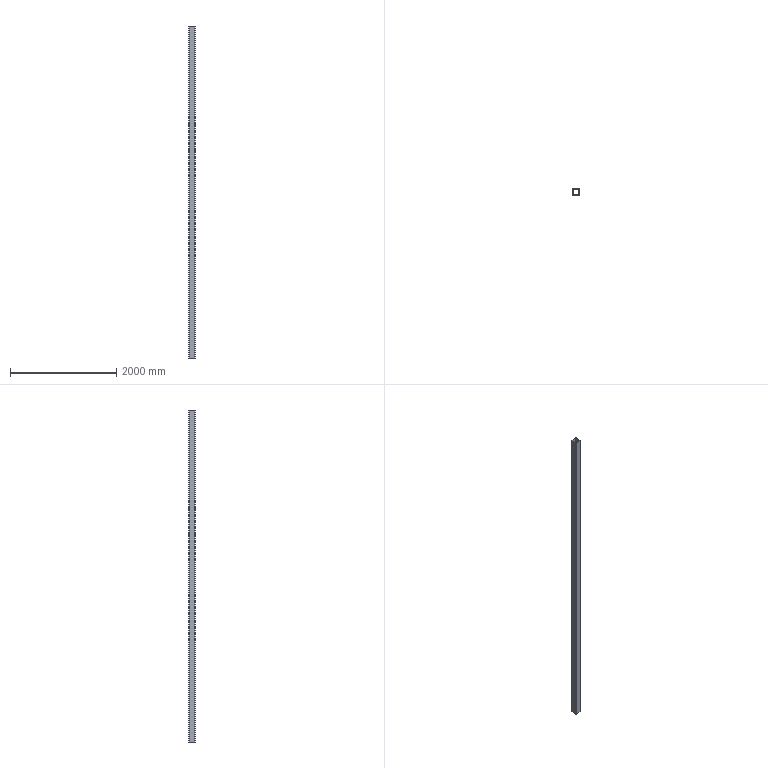Part | SolidWorks | features ICE 1, LibraryFeature 1 | 1 solid | 18 faces | box 120 x 120 x 6260 mm | volume 11360626 mm3 | plane 10 | cylinder 8 | commonest cylinder face diameters 8 x4 16 x4
STEP:
#1=CARTESIAN_POINT('',(52.,60.,-3130.));
#2=VERTEX_POINT('',#1);
#3=CARTESIAN_POINT('',(-52.,60.,-3130.));
#4=VERTEX_POINT('',#3);
#5=CARTESIAN_POINT('',(0.,60.,-3130.));
#6=DIRECTION('',(-1.,0.,0.));
#7=VECTOR('',#6,1000.);
#8=LINE('',#5,#7);
#9=EDGE_CURVE('',#2,#4,#8,.T.);
#10=ORIENTED_EDGE('',*,*,#9,.T.);
#11=CARTESIAN_POINT('',(-52.,60.,3130.));
#12=VERTEX_POINT('',#11);
#13=CARTESIAN_POINT('',(-52.,60.,3130.));
#14=DIRECTION('',(0.,0.,-1.));
#15=VECTOR('',#14,1000.);
#16=LINE('',#13,#15);
#17=EDGE_CURVE('',#12,#4,#16,.T.);
#18=ORIENTED_EDGE('',*,*,#17,.F.);
#19=CARTESIAN_POINT('',(52.,60.,3130.));
#20=VERTEX_POINT('',#19);
#21=CARTESIAN_POINT('',(0.,60.,3130.));
#22=DIRECTION('',(-1.,0.,0.));
#23=VECTOR('',#22,1000.);
#24=LINE('',#21,#23);
#25=EDGE_CURVE('',#20,#12,#24,.T.);
#26=ORIENTED_EDGE('',*,*,#25,.F.);
#27=CARTESIAN_POINT('',(52.,60.,3130.));
#28=DIRECTION('',(0.,0.,-1.));
#29=VECTOR('',#28,1000.);
#30=LINE('',#27,#29);
#31=EDGE_CURVE('',#20,#2,#30,.T.);
#32=ORIENTED_EDGE('',*,*,#31,.T.);
#33=EDGE_LOOP('',(#10,#18,#26,#32));
#34=FACE_OUTER_BOUND('',#33,.T.);
#35=CARTESIAN_POINT('',(0.,60.,3130.));
#36=DIRECTION('',(0.,-1.,0.));
#37=DIRECTION('',(0.,0.,-1.));
#38=AXIS2_PLACEMENT_3D('',#35,#36,#37);
#39=PLANE('',#38);
#40=ADVANCED_FACE('',(#34),#39,.F.);
#41=CARTESIAN_POINT('',(-60.,52.,-3130.));
#42=VERTEX_POINT('',#41);
#43=CARTESIAN_POINT('',(-52.,52.,-3130.));
#44=DIRECTION('',(0.,0.,1.));
#45=DIRECTION('',(1.,0.,0.));
#46=AXIS2_PLACEMENT_3D('',#43,#44,#45);
#47=CIRCLE('',#46,8.);
#48=EDGE_CURVE('',#4,#42,#47,.T.);
#49=ORIENTED_EDGE('',*,*,#48,.T.);
#50=CARTESIAN_POINT('',(-60.,52.,3130.));
#51=VERTEX_POINT('',#50);
#52=CARTESIAN_POINT('',(-60.,52.,3130.));
#53=DIRECTION('',(0.,0.,-1.));
#54=VECTOR('',#53,1000.);
#55=LINE('',#52,#54);
#56=EDGE_CURVE('',#51,#42,#55,.T.);
#57=ORIENTED_EDGE('',*,*,#56,.F.);
#58=CARTESIAN_POINT('',(-52.,52.,3130.));
#59=DIRECTION('',(0.,0.,1.));
#60=DIRECTION('',(1.,0.,0.));
#61=AXIS2_PLACEMENT_3D('',#58,#59,#60);
#62=CIRCLE('',#61,8.);
#63=EDGE_CURVE('',#12,#51,#62,.T.);
#64=ORIENTED_EDGE('',*,*,#63,.F.);
#65=ORIENTED_EDGE('',*,*,#17,.T.);
#66=EDGE_LOOP('',(#49,#57,#64,#65));
#67=FACE_OUTER_BOUND('',#66,.T.);
#68=CARTESIAN_POINT('',(-52.,52.,3130.));
#69=DIRECTION('',(0.,0.,-1.));
#70=DIRECTION('',(-1.,0.,0.));
#71=AXIS2_PLACEMENT_3D('',#68,#69,#70);
#72=CYLINDRICAL_SURFACE('',#71,8.);
#73=ADVANCED_FACE('',(#67),#72,.T.);
#74=CARTESIAN_POINT('',(-60.,-52.,-3130.));
#75=VERTEX_POINT('',#74);
#76=CARTESIAN_POINT('',(-60.,0.,-3130.));
#77=DIRECTION('',(0.,1.,0.));
#78=VECTOR('',#77,1000.);
#79=LINE('',#76,#78);
#80=EDGE_CURVE('',#75,#42,#79,.T.);
#81=ORIENTED_EDGE('',*,*,#80,.F.);
#82=CARTESIAN_POINT('',(-60.,-52.,3130.));
#83=VERTEX_POINT('',#82);
#84=CARTESIAN_POINT('',(-60.,-52.,3130.));
#85=DIRECTION('',(0.,0.,-1.));
#86=VECTOR('',#85,1000.);
#87=LINE('',#84,#86);
#88=EDGE_CURVE('',#83,#75,#87,.T.);
#89=ORIENTED_EDGE('',*,*,#88,.F.);
#90=CARTESIAN_POINT('',(-60.,0.,3130.));
#91=DIRECTION('',(0.,1.,0.));
#92=VECTOR('',#91,1000.);
#93=LINE('',#90,#92);
#94=EDGE_CURVE('',#83,#51,#93,.T.);
#95=ORIENTED_EDGE('',*,*,#94,.T.);
#96=ORIENTED_EDGE('',*,*,#56,.T.);
#97=EDGE_LOOP('',(#81,#89,#95,#96));
#98=FACE_OUTER_BOUND('',#97,.T.);
#99=CARTESIAN_POINT('',(-60.,0.,3130.));
#100=DIRECTION('',(-1.,0.,0.));
#101=DIRECTION('',(0.,0.,1.));
#102=AXIS2_PLACEMENT_3D('',#99,#100,#101);
#103=PLANE('',#102);
#104=ADVANCED_FACE('',(#98),#103,.T.);
#105=CARTESIAN_POINT('',(-52.,-60.,-3130.));
#106=VERTEX_POINT('',#105);
#107=CARTESIAN_POINT('',(-52.,-52.,-3130.));
#108=DIRECTION('',(0.,0.,1.));
#109=DIRECTION('',(1.,0.,0.));
#110=AXIS2_PLACEMENT_3D('',#107,#108,#109);
#111=CIRCLE('',#110,8.);
#112=EDGE_CURVE('',#75,#106,#111,.T.);
#113=ORIENTED_EDGE('',*,*,#112,.T.);
#114=CARTESIAN_POINT('',(-52.,-60.,3130.));
#115=VERTEX_POINT('',#114);
#116=CARTESIAN_POINT('',(-52.,-60.,3130.));
#117=DIRECTION('',(0.,0.,-1.));
#118=VECTOR('',#117,1000.);
#119=LINE('',#116,#118);
#120=EDGE_CURVE('',#115,#106,#119,.T.);
#121=ORIENTED_EDGE('',*,*,#120,.F.);
#122=CARTESIAN_POINT('',(-52.,-52.,3130.));
#123=DIRECTION('',(0.,0.,1.));
#124=DIRECTION('',(1.,0.,0.));
#125=AXIS2_PLACEMENT_3D('',#122,#123,#124);
#126=CIRCLE('',#125,8.);
#127=EDGE_CURVE('',#83,#115,#126,.T.);
#128=ORIENTED_EDGE('',*,*,#127,.F.);
#129=ORIENTED_EDGE('',*,*,#88,.T.);
#130=EDGE_LOOP('',(#113,#121,#128,#129));
#131=FACE_OUTER_BOUND('',#130,.T.);
#132=CARTESIAN_POINT('',(-52.,-52.,3130.));
#133=DIRECTION('',(0.,0.,-1.));
#134=DIRECTION('',(-1.,0.,0.));
#135=AXIS2_PLACEMENT_3D('',#132,#133,#134);
#136=CYLINDRICAL_SURFACE('',#135,8.);
#137=ADVANCED_FACE('',(#131),#136,.T.);
#138=CARTESIAN_POINT('',(52.,-60.,-3130.));
#139=VERTEX_POINT('',#138);
#140=CARTESIAN_POINT('',(0.,-60.,-3130.));
#141=DIRECTION('',(1.,0.,0.));
#142=VECTOR('',#141,1000.);
#143=LINE('',#140,#142);
#144=EDGE_CURVE('',#106,#139,#143,.T.);
#145=ORIENTED_EDGE('',*,*,#144,.T.);
#146=CARTESIAN_POINT('',(52.,-60.,3130.));
#147=VERTEX_POINT('',#146);
#148=CARTESIAN_POINT('',(52.,-60.,3130.));
#149=DIRECTION('',(0.,0.,-1.));
#150=VECTOR('',#149,1000.);
#151=LINE('',#148,#150);
#152=EDGE_CURVE('',#147,#139,#151,.T.);
#153=ORIENTED_EDGE('',*,*,#152,.F.);
#154=CARTESIAN_POINT('',(0.,-60.,3130.));
#155=DIRECTION('',(1.,0.,0.));
#156=VECTOR('',#155,1000.);
#157=LINE('',#154,#156);
#158=EDGE_CURVE('',#115,#147,#157,.T.);
#159=ORIENTED_EDGE('',*,*,#158,.F.);
#160=ORIENTED_EDGE('',*,*,#120,.T.);
#161=EDGE_LOOP('',(#145,#153,#159,#160));
#162=FACE_OUTER_BOUND('',#161,.T.);
#163=CARTESIAN_POINT('',(0.,-60.,3130.));
#164=DIRECTION('',(0.,1.,0.));
#165=DIRECTION('',(0.,0.,1.));
#166=AXIS2_PLACEMENT_3D('',#163,#164,#165);
#167=PLANE('',#166);
#168=ADVANCED_FACE('',(#162),#167,.F.);
#169=CARTESIAN_POINT('',(60.,-52.,-3130.));
#170=VERTEX_POINT('',#169);
#171=CARTESIAN_POINT('',(52.,-52.,-3130.));
#172=DIRECTION('',(0.,0.,1.));
#173=DIRECTION('',(1.,0.,0.));
#174=AXIS2_PLACEMENT_3D('',#171,#172,#173);
#175=CIRCLE('',#174,8.);
#176=EDGE_CURVE('',#139,#170,#175,.T.);
#177=ORIENTED_EDGE('',*,*,#176,.T.);
#178=CARTESIAN_POINT('',(60.,-52.,3130.));
#179=VERTEX_POINT('',#178);
#180=CARTESIAN_POINT('',(60.,-52.,3130.));
#181=DIRECTION('',(0.,0.,-1.));
#182=VECTOR('',#181,1000.);
#183=LINE('',#180,#182);
#184=EDGE_CURVE('',#179,#170,#183,.T.);
#185=ORIENTED_EDGE('',*,*,#184,.F.);
#186=CARTESIAN_POINT('',(52.,-52.,3130.));
#187=DIRECTION('',(0.,0.,1.));
#188=DIRECTION('',(1.,0.,0.));
#189=AXIS2_PLACEMENT_3D('',#186,#187,#188);
#190=CIRCLE('',#189,8.);
#191=EDGE_CURVE('',#147,#179,#190,.T.);
#192=ORIENTED_EDGE('',*,*,#191,.F.);
#193=ORIENTED_EDGE('',*,*,#152,.T.);
#194=EDGE_LOOP('',(#177,#185,#192,#193));
#195=FACE_OUTER_BOUND('',#194,.T.);
#196=CARTESIAN_POINT('',(52.,-52.,3130.));
#197=DIRECTION('',(0.,0.,-1.));
#198=DIRECTION('',(-1.,0.,0.));
#199=AXIS2_PLACEMENT_3D('',#196,#197,#198);
#200=CYLINDRICAL_SURFACE('',#199,8.);
#201=ADVANCED_FACE('',(#195),#200,.T.);
#202=CARTESIAN_POINT('',(60.,52.,-3130.));
#203=VERTEX_POINT('',#202);
#204=CARTESIAN_POINT('',(60.,0.,-3130.));
#205=DIRECTION('',(0.,-1.,0.));
#206=VECTOR('',#205,1000.);
#207=LINE('',#204,#206);
#208=EDGE_CURVE('',#203,#170,#207,.T.);
#209=ORIENTED_EDGE('',*,*,#208,.F.);
#210=CARTESIAN_POINT('',(60.,52.,3130.));
#211=VERTEX_POINT('',#210);
#212=CARTESIAN_POINT('',(60.,52.,3130.));
#213=DIRECTION('',(0.,0.,-1.));
#214=VECTOR('',#213,1000.);
#215=LINE('',#212,#214);
#216=EDGE_CURVE('',#211,#203,#215,.T.);
#217=ORIENTED_EDGE('',*,*,#216,.F.);
#218=CARTESIAN_POINT('',(60.,0.,3130.));
#219=DIRECTION('',(0.,-1.,0.));
#220=VECTOR('',#219,1000.);
#221=LINE('',#218,#220);
#222=EDGE_CURVE('',#211,#179,#221,.T.);
#223=ORIENTED_EDGE('',*,*,#222,.T.);
#224=ORIENTED_EDGE('',*,*,#184,.T.);
#225=EDGE_LOOP('',(#209,#217,#223,#224));
#226=FACE_OUTER_BOUND('',#225,.T.);
#227=CARTESIAN_POINT('',(60.,0.,3130.));
#228=DIRECTION('',(1.,0.,0.));
#229=DIRECTION('',(0.,0.,-1.));
#230=AXIS2_PLACEMENT_3D('',#227,#228,#229);
#231=PLANE('',#230);
#232=ADVANCED_FACE('',(#226),#231,.T.);
#233=CARTESIAN_POINT('',(-56.,-52.,-3130.));
#234=VERTEX_POINT('',#233);
#235=CARTESIAN_POINT('',(-52.,-56.,-3130.));
#236=VERTEX_POINT('',#235);
#237=CARTESIAN_POINT('',(-52.,-52.,-3130.));
#238=DIRECTION('',(0.,0.,1.));
#239=DIRECTION('',(1.,0.,0.));
#240=AXIS2_PLACEMENT_3D('',#237,#238,#239);
#241=CIRCLE('',#240,4.);
#242=EDGE_CURVE('',#234,#236,#241,.T.);
#243=ORIENTED_EDGE('',*,*,#242,.F.);
#244=CARTESIAN_POINT('',(-56.,-52.,3130.));
#245=VERTEX_POINT('',#244);
#246=CARTESIAN_POINT('',(-56.,-52.,3130.));
#247=DIRECTION('',(0.,0.,-1.));
#248=VECTOR('',#247,1000.);
#249=LINE('',#246,#248);
#250=EDGE_CURVE('',#245,#234,#249,.T.);
#251=ORIENTED_EDGE('',*,*,#250,.F.);
#252=CARTESIAN_POINT('',(-52.,-56.,3130.));
#253=VERTEX_POINT('',#252);
#254=CARTESIAN_POINT('',(-52.,-52.,3130.));
#255=DIRECTION('',(0.,0.,1.));
#256=DIRECTION('',(1.,0.,0.));
#257=AXIS2_PLACEMENT_3D('',#254,#255,#256);
#258=CIRCLE('',#257,4.);
#259=EDGE_CURVE('',#245,#253,#258,.T.);
#260=ORIENTED_EDGE('',*,*,#259,.T.);
#261=CARTESIAN_POINT('',(-52.,-56.,3130.));
#262=DIRECTION('',(0.,0.,-1.));
#263=VECTOR('',#262,1000.);
#264=LINE('',#261,#263);
#265=EDGE_CURVE('',#253,#236,#264,.T.);
#266=ORIENTED_EDGE('',*,*,#265,.T.);
#267=EDGE_LOOP('',(#243,#251,#260,#266));
#268=FACE_OUTER_BOUND('',#267,.T.);
#269=CARTESIAN_POINT('',(-52.,-52.,3130.));
#270=DIRECTION('',(0.,0.,-1.));
#271=DIRECTION('',(-1.,0.,0.));
#272=AXIS2_PLACEMENT_3D('',#269,#270,#271);
#273=CYLINDRICAL_SURFACE('',#272,4.);
#274=ADVANCED_FACE('',(#268),#273,.F.);
#275=CARTESIAN_POINT('',(-56.,52.,-3130.));
#276=VERTEX_POINT('',#275);
#277=CARTESIAN_POINT('',(-56.,0.,-3130.));
#278=DIRECTION('',(0.,1.,0.));
#279=VECTOR('',#278,1000.);
#280=LINE('',#277,#279);
#281=EDGE_CURVE('',#234,#276,#280,.T.);
#282=ORIENTED_EDGE('',*,*,#281,.T.);
#283=CARTESIAN_POINT('',(-56.,52.,3130.));
#284=VERTEX_POINT('',#283);
#285=CARTESIAN_POINT('',(-56.,52.,3130.));
#286=DIRECTION('',(0.,0.,-1.));
#287=VECTOR('',#286,1000.);
#288=LINE('',#285,#287);
#289=EDGE_CURVE('',#284,#276,#288,.T.);
#290=ORIENTED_EDGE('',*,*,#289,.F.);
#291=CARTESIAN_POINT('',(-56.,0.,3130.));
#292=DIRECTION('',(0.,1.,0.));
#293=VECTOR('',#292,1000.);
#294=LINE('',#291,#293);
#295=EDGE_CURVE('',#245,#284,#294,.T.);
#296=ORIENTED_EDGE('',*,*,#295,.F.);
#297=ORIENTED_EDGE('',*,*,#250,.T.);
#298=EDGE_LOOP('',(#282,#290,#296,#297));
#299=FACE_OUTER_BOUND('',#298,.T.);
#300=CARTESIAN_POINT('',(-56.,0.,3130.));
#301=DIRECTION('',(-1.,0.,0.));
#302=DIRECTION('',(0.,0.,1.));
#303=AXIS2_PLACEMENT_3D('',#300,#301,#302);
#304=PLANE('',#303);
#305=ADVANCED_FACE('',(#299),#304,.F.);
#306=CARTESIAN_POINT('',(-52.,56.,-3130.));
#307=VERTEX_POINT('',#306);
#308=CARTESIAN_POINT('',(-52.,52.,-3130.));
#309=DIRECTION('',(0.,0.,1.));
#310=DIRECTION('',(1.,0.,0.));
#311=AXIS2_PLACEMENT_3D('',#308,#309,#310);
#312=CIRCLE('',#311,4.);
#313=EDGE_CURVE('',#307,#276,#312,.T.);
#314=ORIENTED_EDGE('',*,*,#313,.F.);
#315=CARTESIAN_POINT('',(-52.,56.,3130.));
#316=VERTEX_POINT('',#315);
#317=CARTESIAN_POINT('',(-52.,56.,3130.));
#318=DIRECTION('',(0.,0.,-1.));
#319=VECTOR('',#318,1000.);
#320=LINE('',#317,#319);
#321=EDGE_CURVE('',#316,#307,#320,.T.);
#322=ORIENTED_EDGE('',*,*,#321,.F.);
#323=CARTESIAN_POINT('',(-52.,52.,3130.));
#324=DIRECTION('',(0.,0.,1.));
#325=DIRECTION('',(1.,0.,0.));
#326=AXIS2_PLACEMENT_3D('',#323,#324,#325);
#327=CIRCLE('',#326,4.);
#328=EDGE_CURVE('',#316,#284,#327,.T.);
#329=ORIENTED_EDGE('',*,*,#328,.T.);
#330=ORIENTED_EDGE('',*,*,#289,.T.);
#331=EDGE_LOOP('',(#314,#322,#329,#330));
#332=FACE_OUTER_BOUND('',#331,.T.);
#333=CARTESIAN_POINT('',(-52.,52.,3130.));
#334=DIRECTION('',(0.,0.,-1.));
#335=DIRECTION('',(-1.,0.,0.));
#336=AXIS2_PLACEMENT_3D('',#333,#334,#335);
#337=CYLINDRICAL_SURFACE('',#336,4.);
#338=ADVANCED_FACE('',(#332),#337,.F.);
#339=CARTESIAN_POINT('',(52.,56.,-3130.));
#340=VERTEX_POINT('',#339);
#341=CARTESIAN_POINT('',(0.,56.,-3130.));
#342=DIRECTION('',(-1.,0.,0.));
#343=VECTOR('',#342,1000.);
#344=LINE('',#341,#343);
#345=EDGE_CURVE('',#340,#307,#344,.T.);
#346=ORIENTED_EDGE('',*,*,#345,.F.);
#347=CARTESIAN_POINT('',(52.,56.,3130.));
#348=VERTEX_POINT('',#347);
#349=CARTESIAN_POINT('',(52.,56.,3130.));
#350=DIRECTION('',(0.,0.,-1.));
#351=VECTOR('',#350,1000.);
#352=LINE('',#349,#351);
#353=EDGE_CURVE('',#348,#340,#352,.T.);
#354=ORIENTED_EDGE('',*,*,#353,.F.);
#355=CARTESIAN_POINT('',(0.,56.,3130.));
#356=DIRECTION('',(-1.,0.,0.));
#357=VECTOR('',#356,1000.);
#358=LINE('',#355,#357);
#359=EDGE_CURVE('',#348,#316,#358,.T.);
#360=ORIENTED_EDGE('',*,*,#359,.T.);
#361=ORIENTED_EDGE('',*,*,#321,.T.);
#362=EDGE_LOOP('',(#346,#354,#360,#361));
#363=FACE_OUTER_BOUND('',#362,.T.);
#364=CARTESIAN_POINT('',(0.,56.,3130.));
#365=DIRECTION('',(0.,-1.,0.));
#366=DIRECTION('',(0.,0.,-1.));
#367=AXIS2_PLACEMENT_3D('',#364,#365,#366);
#368=PLANE('',#367);
#369=ADVANCED_FACE('',(#363),#368,.T.);
#370=CARTESIAN_POINT('',(56.,52.,-3130.));
#371=VERTEX_POINT('',#370);
#372=CARTESIAN_POINT('',(52.,52.,-3130.));
#373=DIRECTION('',(0.,0.,1.));
#374=DIRECTION('',(1.,0.,0.));
#375=AXIS2_PLACEMENT_3D('',#372,#373,#374);
#376=CIRCLE('',#375,4.);
#377=EDGE_CURVE('',#371,#340,#376,.T.);
#378=ORIENTED_EDGE('',*,*,#377,.F.);
#379=CARTESIAN_POINT('',(56.,52.,3130.));
#380=VERTEX_POINT('',#379);
#381=CARTESIAN_POINT('',(56.,52.,3130.));
#382=DIRECTION('',(0.,0.,-1.));
#383=VECTOR('',#382,1000.);
#384=LINE('',#381,#383);
#385=EDGE_CURVE('',#380,#371,#384,.T.);
#386=ORIENTED_EDGE('',*,*,#385,.F.);
#387=CARTESIAN_POINT('',(52.,52.,3130.));
#388=DIRECTION('',(0.,0.,1.));
#389=DIRECTION('',(1.,0.,0.));
#390=AXIS2_PLACEMENT_3D('',#387,#388,#389);
#391=CIRCLE('',#390,4.);
#392=EDGE_CURVE('',#380,#348,#391,.T.);
#393=ORIENTED_EDGE('',*,*,#392,.T.);
#394=ORIENTED_EDGE('',*,*,#353,.T.);
#395=EDGE_LOOP('',(#378,#386,#393,#394));
#396=FACE_OUTER_BOUND('',#395,.T.);
#397=CARTESIAN_POINT('',(52.,52.,3130.));
#398=DIRECTION('',(0.,0.,-1.));
#399=DIRECTION('',(-1.,0.,0.));
#400=AXIS2_PLACEMENT_3D('',#397,#398,#399);
#401=CYLINDRICAL_SURFACE('',#400,4.);
#402=ADVANCED_FACE('',(#396),#401,.F.);
#403=CARTESIAN_POINT('',(56.,-52.,-3130.));
#404=VERTEX_POINT('',#403);
#405=CARTESIAN_POINT('',(56.,0.,-3130.));
#406=DIRECTION('',(0.,-1.,0.));
#407=VECTOR('',#406,1000.);
#408=LINE('',#405,#407);
#409=EDGE_CURVE('',#371,#404,#408,.T.);
#410=ORIENTED_EDGE('',*,*,#409,.T.);
#411=CARTESIAN_POINT('',(56.,-52.,3130.));
#412=VERTEX_POINT('',#411);
#413=CARTESIAN_POINT('',(56.,-52.,3130.));
#414=DIRECTION('',(0.,0.,-1.));
#415=VECTOR('',#414,1000.);
#416=LINE('',#413,#415);
#417=EDGE_CURVE('',#412,#404,#416,.T.);
#418=ORIENTED_EDGE('',*,*,#417,.F.);
#419=CARTESIAN_POINT('',(56.,0.,3130.));
#420=DIRECTION('',(0.,-1.,0.));
#421=VECTOR('',#420,1000.);
#422=LINE('',#419,#421);
#423=EDGE_CURVE('',#380,#412,#422,.T.);
#424=ORIENTED_EDGE('',*,*,#423,.F.);
#425=ORIENTED_EDGE('',*,*,#385,.T.);
#426=EDGE_LOOP('',(#410,#418,#424,#425));
#427=FACE_OUTER_BOUND('',#426,.T.);
#428=CARTESIAN_POINT('',(56.,0.,3130.));
#429=DIRECTION('',(1.,0.,0.));
#430=DIRECTION('',(0.,0.,-1.));
#431=AXIS2_PLACEMENT_3D('',#428,#429,#430);
#432=PLANE('',#431);
#433=ADVANCED_FACE('',(#427),#432,.F.);
#434=CARTESIAN_POINT('',(52.,-56.,-3130.));
#435=VERTEX_POINT('',#434);
#436=CARTESIAN_POINT('',(52.,-52.,-3130.));
#437=DIRECTION('',(0.,0.,1.));
#438=DIRECTION('',(1.,0.,0.));
#439=AXIS2_PLACEMENT_3D('',#436,#437,#438);
#440=CIRCLE('',#439,4.);
#441=EDGE_CURVE('',#435,#404,#440,.T.);
#442=ORIENTED_EDGE('',*,*,#441,.F.);
#443=CARTESIAN_POINT('',(52.,-56.,3130.));
#444=VERTEX_POINT('',#443);
#445=CARTESIAN_POINT('',(52.,-56.,3130.));
#446=DIRECTION('',(0.,0.,-1.));
#447=VECTOR('',#446,1000.);
#448=LINE('',#445,#447);
#449=EDGE_CURVE('',#444,#435,#448,.T.);
#450=ORIENTED_EDGE('',*,*,#449,.F.);
#451=CARTESIAN_POINT('',(52.,-52.,3130.));
#452=DIRECTION('',(0.,0.,1.));
#453=DIRECTION('',(1.,0.,0.));
#454=AXIS2_PLACEMENT_3D('',#451,#452,#453);
#455=CIRCLE('',#454,4.);
#456=EDGE_CURVE('',#444,#412,#455,.T.);
#457=ORIENTED_EDGE('',*,*,#456,.T.);
#458=ORIENTED_EDGE('',*,*,#417,.T.);
#459=EDGE_LOOP('',(#442,#450,#457,#458));
#460=FACE_OUTER_BOUND('',#459,.T.);
#461=CARTESIAN_POINT('',(52.,-52.,3130.));
#462=DIRECTION('',(0.,0.,-1.));
#463=DIRECTION('',(-1.,0.,0.));
#464=AXIS2_PLACEMENT_3D('',#461,#462,#463);
#465=CYLINDRICAL_SURFACE('',#464,4.);
#466=ADVANCED_FACE('',(#460),#465,.F.);
#467=CARTESIAN_POINT('',(0.,-56.,-3130.));
#468=DIRECTION('',(1.,0.,0.));
#469=VECTOR('',#468,1000.);
#470=LINE('',#467,#469);
#471=EDGE_CURVE('',#236,#435,#470,.T.);
#472=ORIENTED_EDGE('',*,*,#471,.F.);
#473=ORIENTED_EDGE('',*,*,#265,.F.);
#474=CARTESIAN_POINT('',(0.,-56.,3130.));
#475=DIRECTION('',(1.,0.,0.));
#476=VECTOR('',#475,1000.);
#477=LINE('',#474,#476);
#478=EDGE_CURVE('',#253,#444,#477,.T.);
#479=ORIENTED_EDGE('',*,*,#478,.T.);
#480=ORIENTED_EDGE('',*,*,#449,.T.);
#481=EDGE_LOOP('',(#472,#473,#479,#480));
#482=FACE_OUTER_BOUND('',#481,.T.);
#483=CARTESIAN_POINT('',(0.,-56.,3130.));
#484=DIRECTION('',(0.,1.,0.));
#485=DIRECTION('',(0.,0.,1.));
#486=AXIS2_PLACEMENT_3D('',#483,#484,#485);
#487=PLANE('',#486);
#488=ADVANCED_FACE('',(#482),#487,.T.);
#489=CARTESIAN_POINT('',(52.,52.,-3130.));
#490=DIRECTION('',(0.,0.,1.));
#491=DIRECTION('',(1.,0.,0.));
#492=AXIS2_PLACEMENT_3D('',#489,#490,#491);
#493=CIRCLE('',#492,8.);
#494=EDGE_CURVE('',#203,#2,#493,.T.);
#495=ORIENTED_EDGE('',*,*,#494,.T.);
#496=ORIENTED_EDGE('',*,*,#31,.F.);
#497=CARTESIAN_POINT('',(52.,52.,3130.));
#498=DIRECTION('',(0.,0.,1.));
#499=DIRECTION('',(1.,0.,0.));
#500=AXIS2_PLACEMENT_3D('',#497,#498,#499);
#501=CIRCLE('',#500,8.);
#502=EDGE_CURVE('',#211,#20,#501,.T.);
#503=ORIENTED_EDGE('',*,*,#502,.F.);
#504=ORIENTED_EDGE('',*,*,#216,.T.);
#505=EDGE_LOOP('',(#495,#496,#503,#504));
#506=FACE_OUTER_BOUND('',#505,.T.);
#507=CARTESIAN_POINT('',(52.,52.,3130.));
#508=DIRECTION('',(0.,0.,-1.));
#509=DIRECTION('',(-1.,0.,0.));
#510=AXIS2_PLACEMENT_3D('',#507,#508,#509);
#511=CYLINDRICAL_SURFACE('',#510,8.);
#512=ADVANCED_FACE('',(#506),#511,.T.);
#513=ORIENTED_EDGE('',*,*,#259,.F.);
#514=ORIENTED_EDGE('',*,*,#295,.T.);
#515=ORIENTED_EDGE('',*,*,#328,.F.);
#516=ORIENTED_EDGE('',*,*,#359,.F.);
#517=ORIENTED_EDGE('',*,*,#392,.F.);
#518=ORIENTED_EDGE('',*,*,#423,.T.);
#519=ORIENTED_EDGE('',*,*,#456,.F.);
#520=ORIENTED_EDGE('',*,*,#478,.F.);
#521=EDGE_LOOP('',(#513,#514,#515,#516,#517,#518,#519,#520));
#522=FACE_BOUND('',#521,.T.);
#523=ORIENTED_EDGE('',*,*,#25,.T.);
#524=ORIENTED_EDGE('',*,*,#63,.T.);
#525=ORIENTED_EDGE('',*,*,#94,.F.);
#526=ORIENTED_EDGE('',*,*,#127,.T.);
#527=ORIENTED_EDGE('',*,*,#158,.T.);
#528=ORIENTED_EDGE('',*,*,#191,.T.);
#529=ORIENTED_EDGE('',*,*,#222,.F.);
#530=ORIENTED_EDGE('',*,*,#502,.T.);
#531=EDGE_LOOP('',(#523,#524,#525,#526,#527,#528,#529,#530));
#532=FACE_OUTER_BOUND('',#531,.T.);
#533=CARTESIAN_POINT('',(0.,0.,3130.));
#534=DIRECTION('',(0.,0.,1.));
#535=DIRECTION('',(1.,0.,0.));
#536=AXIS2_PLACEMENT_3D('',#533,#534,#535);
#537=PLANE('',#536);
#538=ADVANCED_FACE('',(#522,#532),#537,.T.);
#539=ORIENTED_EDGE('',*,*,#242,.T.);
#540=ORIENTED_EDGE('',*,*,#471,.T.);
#541=ORIENTED_EDGE('',*,*,#441,.T.);
#542=ORIENTED_EDGE('',*,*,#409,.F.);
#543=ORIENTED_EDGE('',*,*,#377,.T.);
#544=ORIENTED_EDGE('',*,*,#345,.T.);
#545=ORIENTED_EDGE('',*,*,#313,.T.);
#546=ORIENTED_EDGE('',*,*,#281,.F.);
#547=EDGE_LOOP('',(#539,#540,#541,#542,#543,#544,#545,#546));
#548=FACE_BOUND('',#547,.T.);
#549=ORIENTED_EDGE('',*,*,#9,.F.);
#550=ORIENTED_EDGE('',*,*,#494,.F.);
#551=ORIENTED_EDGE('',*,*,#208,.T.);
#552=ORIENTED_EDGE('',*,*,#176,.F.);
#553=ORIENTED_EDGE('',*,*,#144,.F.);
#554=ORIENTED_EDGE('',*,*,#112,.F.);
#555=ORIENTED_EDGE('',*,*,#80,.T.);
#556=ORIENTED_EDGE('',*,*,#48,.F.);
#557=EDGE_LOOP('',(#549,#550,#551,#552,#553,#554,#555,#556));
#558=FACE_OUTER_BOUND('',#557,.T.);
#559=CARTESIAN_POINT('',(0.,0.,-3130.));
#560=DIRECTION('',(0.,0.,1.));
#561=DIRECTION('',(1.,0.,0.));
#562=AXIS2_PLACEMENT_3D('',#559,#560,#561);
#563=PLANE('',#562);
#564=ADVANCED_FACE('',(#548,#558),#563,.F.);
#565=CLOSED_SHELL('',(#40,#73,#104,#137,#168,#201,#232,#274,#305,#338,#369,#402,#433,#466,#488,#512,#538,#564));
#566=MANIFOLD_SOLID_BREP('',#565);
#567=CARTESIAN_POINT('',(0.,0.,0.));
#568=DIRECTION('',(0.,0.,1.));
#569=DIRECTION('',(1.,0.,0.));
#570=AXIS2_PLACEMENT_3D('',#567,#568,#569);
#571=(LENGTH_UNIT()NAMED_UNIT(*)SI_UNIT(.MILLI.,.METRE.));
#572=UNCERTAINTY_MEASURE_WITH_UNIT(LENGTH_MEASURE(0.00001),#571,'','');
#573=(NAMED_UNIT(*)PLANE_ANGLE_UNIT()SI_UNIT($,.RADIAN.));
#574=(NAMED_UNIT(*)SI_UNIT($,.STERADIAN.)SOLID_ANGLE_UNIT());
#575=(GEOMETRIC_REPRESENTATION_CONTEXT(3)GLOBAL_UNCERTAINTY_ASSIGNED_CONTEXT((#572))GLOBAL_UNIT_ASSIGNED_CONTEXT((#571,#573,#574))REPRESENTATION_CONTEXT('',''));
#576=ADVANCED_BREP_SHAPE_REPRESENTATION('',(#566,#570),#575);